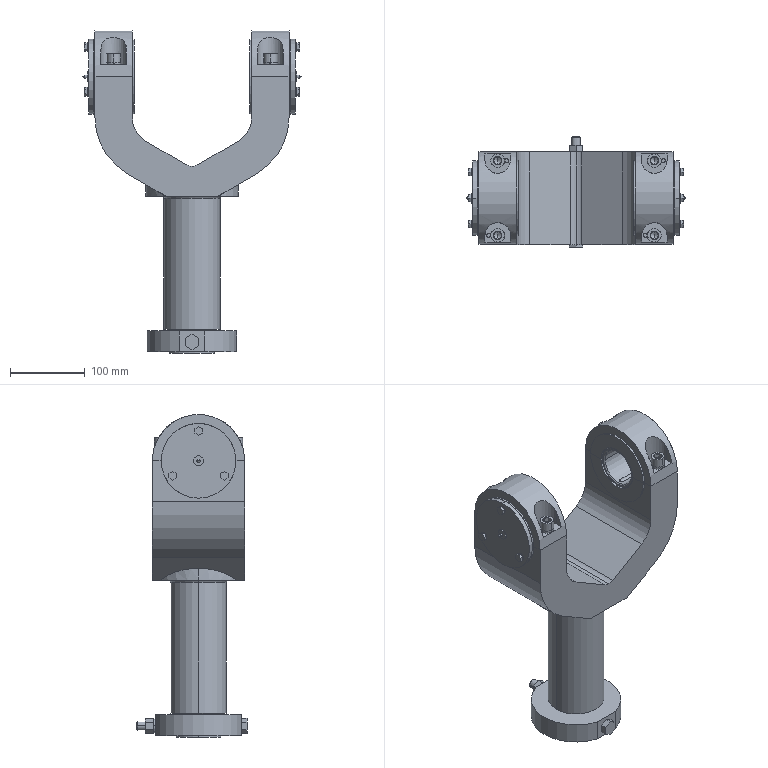Part | SolidWorks | features ReferencePattern 21, MirrorCompFeat 4, LocalCirPattern 1, LocalLPattern 1 | 37 solids | 599 faces | box 292 x 147.5 x 432 mm | volume 4101451 mm3 | plane 246 | cylinder 217 | cone 126 | sphere 8 | torus 2 | commonest cylinder face diameters 6 x38 12.2 x15 18.4 x15 13 x14 5 x12 6.1 x12